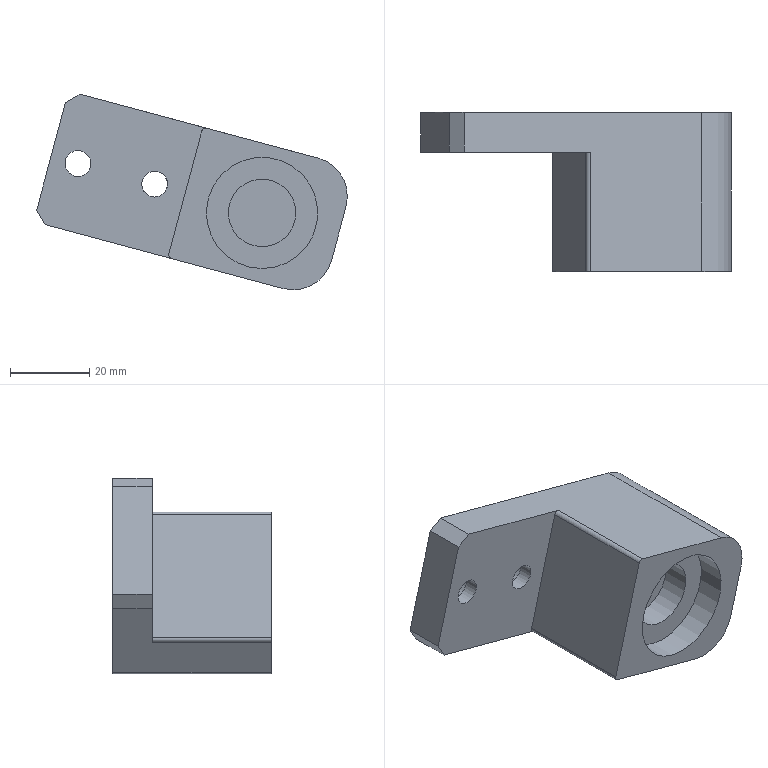Part | NX | 1 solid | 24 faces | box 78.22 x 40 x 49.229 mm | volume 57101 mm3 | plane 14 | cylinder 10 | commonest cylinder face diameters 2 x2 6.5 x2 11 x2 20 x2 17 x1 28.04 x1
STEP:
#1=CARTESIAN_POINT('',(554.778,70.097,-14.611));
#2=VERTEX_POINT('',#1);
#3=CARTESIAN_POINT('',(554.778,70.097,-0.5914));
#4=DIRECTION('',(0.,1.,0.));
#5=DIRECTION('',(0.000000051,0.,-1.));
#6=AXIS2_PLACEMENT_3D('',#3,#4,#5);
#7=CIRCLE('',#6,14.02);
#8=EDGE_CURVE('',#2,#2,#7,.T.);
#9=ORIENTED_EDGE('',*,*,#8,.F.);
#10=EDGE_LOOP('',(#9));
#11=FACE_BOUND('',#10,.T.);
#12=CARTESIAN_POINT('',(554.778,70.097,7.909));
#13=VERTEX_POINT('',#12);
#14=CARTESIAN_POINT('',(554.778,70.097,-0.5914));
#15=DIRECTION('',(0.,1.,0.));
#16=DIRECTION('',(0.,0.,1.));
#17=AXIS2_PLACEMENT_3D('',#14,#15,#16);
#18=CIRCLE('',#17,8.5);
#19=EDGE_CURVE('',#13,#13,#18,.T.);
#20=ORIENTED_EDGE('',*,*,#19,.T.);
#21=EDGE_LOOP('',(#20));
#22=FACE_BOUND('',#21,.T.);
#23=CARTESIAN_POINT('',(554.778,70.097,-0.5914));
#24=DIRECTION('',(0.,1.,0.));
#25=DIRECTION('',(0.9659,0.,-0.2588));
#26=AXIS2_PLACEMENT_3D('',#23,#24,#25);
#27=PLANE('',#26);
#28=ADVANCED_FACE('',(#11,#22),#27,.F.);
#29=CARTESIAN_POINT('',(508.413,103.097,17.332));
#30=VERTEX_POINT('',#29);
#31=CARTESIAN_POINT('',(508.413,103.097,11.832));
#32=DIRECTION('',(0.,1.,0.));
#33=DIRECTION('',(0.,0.,1.));
#34=AXIS2_PLACEMENT_3D('',#31,#32,#33);
#35=CIRCLE('',#34,5.5);
#36=EDGE_CURVE('',#30,#30,#35,.T.);
#37=ORIENTED_EDGE('',*,*,#36,.F.);
#38=EDGE_LOOP('',(#37));
#39=FACE_BOUND('',#38,.T.);
#40=CARTESIAN_POINT('',(527.732,103.097,12.156));
#41=VERTEX_POINT('',#40);
#42=CARTESIAN_POINT('',(527.732,103.097,6.656));
#43=DIRECTION('',(0.,1.,0.));
#44=DIRECTION('',(0.,0.,1.));
#45=AXIS2_PLACEMENT_3D('',#42,#43,#44);
#46=CIRCLE('',#45,5.5);
#47=EDGE_CURVE('',#41,#41,#46,.T.);
#48=ORIENTED_EDGE('',*,*,#47,.F.);
#49=EDGE_LOOP('',(#48));
#50=FACE_BOUND('',#49,.T.);
#51=CARTESIAN_POINT('',(498.028,103.097,0.1207));
#52=VERTEX_POINT('',#51);
#53=CARTESIAN_POINT('',(500.15,103.097,-3.554));
#54=VERTEX_POINT('',#53);
#55=CARTESIAN_POINT('',(500.15,103.097,-3.554));
#56=DIRECTION('',(0.5,0.,-0.866));
#57=VECTOR('',#56,1000.);
#58=LINE('',#55,#57);
#59=EDGE_CURVE('',#52,#54,#58,.T.);
#60=ORIENTED_EDGE('',*,*,#59,.F.);
#61=CARTESIAN_POINT('',(505.275,103.097,27.167));
#62=VERTEX_POINT('',#61);
#63=CARTESIAN_POINT('',(501.652,103.097,13.644));
#64=DIRECTION('',(0.2588,0.,0.9659));
#65=VECTOR('',#64,1000.);
#66=LINE('',#63,#65);
#67=EDGE_CURVE('',#52,#62,#66,.T.);
#68=ORIENTED_EDGE('',*,*,#67,.T.);
#69=CARTESIAN_POINT('',(508.95,103.097,29.288));
#70=VERTEX_POINT('',#69);
#71=CARTESIAN_POINT('',(505.275,103.097,27.167));
#72=DIRECTION('',(-0.866,0.,-0.5));
#73=VECTOR('',#72,1000.);
#74=LINE('',#71,#73);
#75=EDGE_CURVE('',#70,#62,#74,.T.);
#76=ORIENTED_EDGE('',*,*,#75,.F.);
#77=CARTESIAN_POINT('',(568.837,103.097,13.241));
#78=VERTEX_POINT('',#77);
#79=CARTESIAN_POINT('',(342.81,103.097,73.805));
#80=DIRECTION('',(-0.9659,0.,0.2588));
#81=VECTOR('',#80,1000.);
#82=LINE('',#79,#81);
#83=EDGE_CURVE('',#78,#70,#82,.T.);
#84=ORIENTED_EDGE('',*,*,#83,.F.);
#85=CARTESIAN_POINT('',(575.908,103.097,0.9937));
#86=VERTEX_POINT('',#85);
#87=CARTESIAN_POINT('',(566.249,103.097,3.582));
#88=DIRECTION('',(0.,1.,0.));
#89=DIRECTION('',(0.,0.,1.));
#90=AXIS2_PLACEMENT_3D('',#87,#88,#89);
#91=CIRCLE('',#90,10.);
#92=EDGE_CURVE('',#86,#78,#91,.F.);
#93=ORIENTED_EDGE('',*,*,#92,.F.);
#94=CARTESIAN_POINT('',(572.285,103.097,-12.529));
#95=VERTEX_POINT('',#94);
#96=CARTESIAN_POINT('',(572.802,103.097,-10.597));
#97=DIRECTION('',(0.2588,0.,0.9659));
#98=VECTOR('',#97,1000.);
#99=LINE('',#96,#98);
#100=EDGE_CURVE('',#95,#86,#99,.T.);
#101=ORIENTED_EDGE('',*,*,#100,.F.);
#102=CARTESIAN_POINT('',(560.037,103.097,-19.6));
#103=VERTEX_POINT('',#102);
#104=CARTESIAN_POINT('',(562.625,103.097,-9.941));
#105=DIRECTION('',(0.,1.,0.));
#106=DIRECTION('',(0.,0.,1.));
#107=AXIS2_PLACEMENT_3D('',#104,#105,#106);
#108=CIRCLE('',#107,10.);
#109=EDGE_CURVE('',#103,#95,#108,.F.);
#110=ORIENTED_EDGE('',*,*,#109,.F.);
#111=CARTESIAN_POINT('',(334.01,103.097,40.963));
#112=DIRECTION('',(0.9659,0.,-0.2588));
#113=VECTOR('',#112,1000.);
#114=LINE('',#111,#113);
#115=EDGE_CURVE('',#54,#103,#114,.T.);
#116=ORIENTED_EDGE('',*,*,#115,.F.);
#117=EDGE_LOOP('',(#60,#68,#76,#84,#93,#101,#110,#116));
#118=FACE_BOUND('',#117,.T.);
#119=CARTESIAN_POINT('',(334.528,103.097,42.895));
#120=DIRECTION('',(0.,1.,0.));
#121=DIRECTION('',(0.2588,0.,0.9659));
#122=AXIS2_PLACEMENT_3D('',#119,#120,#121);
#123=PLANE('',#122);
#124=ADVANCED_FACE('',(#39,#50,#118),#123,.T.);
#125=CARTESIAN_POINT('',(560.037,63.097,-19.6));
#126=VERTEX_POINT('',#125);
#127=CARTESIAN_POINT('',(560.037,78.097,-19.6));
#128=DIRECTION('',(0.,1.,0.));
#129=VECTOR('',#128,1000.);
#130=LINE('',#127,#129);
#131=EDGE_CURVE('',#126,#103,#130,.T.);
#132=ORIENTED_EDGE('',*,*,#131,.T.);
#133=ORIENTED_EDGE('',*,*,#109,.T.);
#134=CARTESIAN_POINT('',(572.285,63.097,-12.529));
#135=VERTEX_POINT('',#134);
#136=CARTESIAN_POINT('',(572.285,80.097,-12.529));
#137=DIRECTION('',(0.,-1.,0.));
#138=VECTOR('',#137,1000.);
#139=LINE('',#136,#138);
#140=EDGE_CURVE('',#95,#135,#139,.T.);
#141=ORIENTED_EDGE('',*,*,#140,.T.);
#142=CARTESIAN_POINT('',(562.625,63.097,-9.941));
#143=DIRECTION('',(0.,-1.,0.));
#144=DIRECTION('',(0.,0.,-1.));
#145=AXIS2_PLACEMENT_3D('',#142,#143,#144);
#146=CIRCLE('',#145,10.);
#147=EDGE_CURVE('',#135,#126,#146,.F.);
#148=ORIENTED_EDGE('',*,*,#147,.T.);
#149=EDGE_LOOP('',(#132,#133,#141,#148));
#150=FACE_BOUND('',#149,.T.);
#151=CARTESIAN_POINT('',(562.625,80.097,-9.941));
#152=DIRECTION('',(0.,1.,0.));
#153=DIRECTION('',(-0.9659,0.,0.2588));
#154=AXIS2_PLACEMENT_3D('',#151,#152,#153);
#155=CYLINDRICAL_SURFACE('',#154,10.);
#156=ADVANCED_FACE('',(#150),#155,.T.);
#157=CARTESIAN_POINT('',(532.025,63.097,-12.095));
#158=VERTEX_POINT('',#157);
#159=CARTESIAN_POINT('',(532.025,93.097,-12.095));
#160=VERTEX_POINT('',#159);
#161=CARTESIAN_POINT('',(532.025,93.097,-12.095));
#162=DIRECTION('',(0.,1.,0.));
#163=VECTOR('',#162,1000.);
#164=LINE('',#161,#163);
#165=EDGE_CURVE('',#158,#160,#164,.T.);
#166=ORIENTED_EDGE('',*,*,#165,.T.);
#167=CARTESIAN_POINT('',(500.15,93.097,-3.554));
#168=VERTEX_POINT('',#167);
#169=CARTESIAN_POINT('',(334.01,93.097,40.963));
#170=DIRECTION('',(0.9659,0.,-0.2588));
#171=VECTOR('',#170,1000.);
#172=LINE('',#169,#171);
#173=EDGE_CURVE('',#168,#160,#172,.T.);
#174=ORIENTED_EDGE('',*,*,#173,.F.);
#175=CARTESIAN_POINT('',(500.15,78.097,-3.554));
#176=DIRECTION('',(0.,-1.,0.));
#177=VECTOR('',#176,1000.);
#178=LINE('',#175,#177);
#179=EDGE_CURVE('',#54,#168,#178,.T.);
#180=ORIENTED_EDGE('',*,*,#179,.F.);
#181=ORIENTED_EDGE('',*,*,#115,.T.);
#182=ORIENTED_EDGE('',*,*,#131,.F.);
#183=CARTESIAN_POINT('',(334.01,63.097,40.963));
#184=DIRECTION('',(-0.9659,0.,0.2588));
#185=VECTOR('',#184,1000.);
#186=LINE('',#183,#185);
#187=EDGE_CURVE('',#126,#158,#186,.T.);
#188=ORIENTED_EDGE('',*,*,#187,.T.);
#189=EDGE_LOOP('',(#166,#174,#180,#181,#182,#188));
#190=FACE_BOUND('',#189,.T.);
#191=CARTESIAN_POINT('',(334.01,78.097,40.963));
#192=DIRECTION('',(-0.2588,0.,-0.9659));
#193=DIRECTION('',(0.,1.,0.));
#194=AXIS2_PLACEMENT_3D('',#191,#192,#193);
#195=PLANE('',#194);
#196=ADVANCED_FACE('',(#190),#195,.T.);
#197=ORIENTED_EDGE('',*,*,#165,.F.);
#198=CARTESIAN_POINT('',(531.318,63.097,-10.87));
#199=VERTEX_POINT('',#198);
#200=CARTESIAN_POINT('',(532.284,63.097,-11.129));
#201=DIRECTION('',(0.,-1.,0.));
#202=DIRECTION('',(0.,0.,-1.));
#203=AXIS2_PLACEMENT_3D('',#200,#201,#202);
#204=CIRCLE('',#203,1.);
#205=EDGE_CURVE('',#158,#199,#204,.F.);
#206=ORIENTED_EDGE('',*,*,#205,.T.);
#207=CARTESIAN_POINT('',(531.318,93.097,-10.87));
#208=VERTEX_POINT('',#207);
#209=CARTESIAN_POINT('',(531.318,63.097,-10.87));
#210=DIRECTION('',(0.,-1.,0.));
#211=VECTOR('',#210,1000.);
#212=LINE('',#209,#211);
#213=EDGE_CURVE('',#208,#199,#212,.T.);
#214=ORIENTED_EDGE('',*,*,#213,.F.);
#215=CARTESIAN_POINT('',(532.284,93.097,-11.129));
#216=DIRECTION('',(0.,1.,0.));
#217=DIRECTION('',(0.000000051,0.,-1.));
#218=AXIS2_PLACEMENT_3D('',#215,#216,#217);
#219=CIRCLE('',#218,1.);
#220=EDGE_CURVE('',#160,#208,#219,.T.);
#221=ORIENTED_EDGE('',*,*,#220,.F.);
#222=EDGE_LOOP('',(#197,#206,#214,#221));
#223=FACE_BOUND('',#222,.T.);
#224=CARTESIAN_POINT('',(532.284,70.097,-11.129));
#225=DIRECTION('',(0.,1.,0.));
#226=DIRECTION('',(0.000000051,0.,-1.));
#227=AXIS2_PLACEMENT_3D('',#224,#225,#226);
#228=CYLINDRICAL_SURFACE('',#227,1.);
#229=ADVANCED_FACE('',(#223),#228,.T.);
#230=CARTESIAN_POINT('',(539.6,63.097,20.04));
#231=VERTEX_POINT('',#230);
#232=CARTESIAN_POINT('',(535.459,63.097,4.585));
#233=DIRECTION('',(-0.2588,0.,-0.9659));
#234=VECTOR('',#233,1000.);
#235=LINE('',#232,#234);
#236=EDGE_CURVE('',#231,#199,#235,.T.);
#237=ORIENTED_EDGE('',*,*,#236,.F.);
#238=CARTESIAN_POINT('',(539.6,93.097,20.04));
#239=VERTEX_POINT('',#238);
#240=CARTESIAN_POINT('',(539.6,93.097,20.04));
#241=DIRECTION('',(0.,1.,0.));
#242=VECTOR('',#241,1000.);
#243=LINE('',#240,#242);
#244=EDGE_CURVE('',#231,#239,#243,.T.);
#245=ORIENTED_EDGE('',*,*,#244,.T.);
#246=CARTESIAN_POINT('',(535.459,93.097,4.585));
#247=DIRECTION('',(-0.2588,0.,-0.9659));
#248=VECTOR('',#247,1000.);
#249=LINE('',#246,#248);
#250=EDGE_CURVE('',#239,#208,#249,.T.);
#251=ORIENTED_EDGE('',*,*,#250,.T.);
#252=ORIENTED_EDGE('',*,*,#213,.T.);
#253=EDGE_LOOP('',(#237,#245,#251,#252));
#254=FACE_BOUND('',#253,.T.);
#255=CARTESIAN_POINT('',(535.459,70.097,4.585));
#256=DIRECTION('',(0.9659,0.,-0.2588));
#257=DIRECTION('',(0.2588,0.,0.9659));
#258=AXIS2_PLACEMENT_3D('',#255,#256,#257);
#259=PLANE('',#258);
#260=ADVANCED_FACE('',(#254),#259,.F.);
#261=ORIENTED_EDGE('',*,*,#244,.F.);
#262=CARTESIAN_POINT('',(540.825,63.097,20.747));
#263=VERTEX_POINT('',#262);
#264=CARTESIAN_POINT('',(540.566,63.097,19.781));
#265=DIRECTION('',(0.,-1.,0.));
#266=DIRECTION('',(0.,0.,-1.));
#267=AXIS2_PLACEMENT_3D('',#264,#265,#266);
#268=CIRCLE('',#267,1.);
#269=EDGE_CURVE('',#231,#263,#268,.F.);
#270=ORIENTED_EDGE('',*,*,#269,.T.);
#271=CARTESIAN_POINT('',(540.825,93.097,20.747));
#272=VERTEX_POINT('',#271);
#273=CARTESIAN_POINT('',(540.825,63.097,20.747));
#274=DIRECTION('',(0.,-1.,0.));
#275=VECTOR('',#274,1000.);
#276=LINE('',#273,#275);
#277=EDGE_CURVE('',#272,#263,#276,.T.);
#278=ORIENTED_EDGE('',*,*,#277,.F.);
#279=CARTESIAN_POINT('',(540.566,93.097,19.781));
#280=DIRECTION('',(0.,1.,0.));
#281=DIRECTION('',(0.000000051,0.,-1.));
#282=AXIS2_PLACEMENT_3D('',#279,#280,#281);
#283=CIRCLE('',#282,1.);
#284=EDGE_CURVE('',#239,#272,#283,.T.);
#285=ORIENTED_EDGE('',*,*,#284,.F.);
#286=EDGE_LOOP('',(#261,#270,#278,#285));
#287=FACE_BOUND('',#286,.T.);
#288=CARTESIAN_POINT('',(540.566,78.097,19.781));
#289=DIRECTION('',(0.,1.,0.));
#290=DIRECTION('',(0.000000051,0.,-1.));
#291=AXIS2_PLACEMENT_3D('',#288,#289,#290);
#292=CYLINDRICAL_SURFACE('',#291,1.);
#293=ADVANCED_FACE('',(#287),#292,.T.);
#294=CARTESIAN_POINT('',(508.95,93.097,29.288));
#295=VERTEX_POINT('',#294);
#296=CARTESIAN_POINT('',(342.81,93.097,73.805));
#297=DIRECTION('',(-0.9659,0.,0.2588));
#298=VECTOR('',#297,1000.);
#299=LINE('',#296,#298);
#300=EDGE_CURVE('',#272,#295,#299,.T.);
#301=ORIENTED_EDGE('',*,*,#300,.F.);
#302=ORIENTED_EDGE('',*,*,#277,.T.);
#303=CARTESIAN_POINT('',(568.837,63.097,13.241));
#304=VERTEX_POINT('',#303);
#305=CARTESIAN_POINT('',(342.81,63.097,73.805));
#306=DIRECTION('',(0.9659,0.,-0.2588));
#307=VECTOR('',#306,1000.);
#308=LINE('',#305,#307);
#309=EDGE_CURVE('',#263,#304,#308,.T.);
#310=ORIENTED_EDGE('',*,*,#309,.T.);
#311=CARTESIAN_POINT('',(568.837,78.097,13.241));
#312=DIRECTION('',(0.,-1.,0.));
#313=VECTOR('',#312,1000.);
#314=LINE('',#311,#313);
#315=EDGE_CURVE('',#78,#304,#314,.T.);
#316=ORIENTED_EDGE('',*,*,#315,.F.);
#317=ORIENTED_EDGE('',*,*,#83,.T.);
#318=CARTESIAN_POINT('',(508.95,70.097,29.288));
#319=DIRECTION('',(0.,1.,0.));
#320=VECTOR('',#319,1000.);
#321=LINE('',#318,#320);
#322=EDGE_CURVE('',#295,#70,#321,.T.);
#323=ORIENTED_EDGE('',*,*,#322,.F.);
#324=EDGE_LOOP('',(#301,#302,#310,#316,#317,#323));
#325=FACE_BOUND('',#324,.T.);
#326=CARTESIAN_POINT('',(342.81,78.097,73.805));
#327=DIRECTION('',(0.2588,0.,0.9659));
#328=DIRECTION('',(0.,-1.,0.));
#329=AXIS2_PLACEMENT_3D('',#326,#327,#328);
#330=PLANE('',#329);
#331=ADVANCED_FACE('',(#325),#330,.T.);
#332=CARTESIAN_POINT('',(575.908,63.097,0.9937));
#333=VERTEX_POINT('',#332);
#334=CARTESIAN_POINT('',(575.908,80.097,0.9937));
#335=DIRECTION('',(0.,1.,0.));
#336=VECTOR('',#335,1000.);
#337=LINE('',#334,#336);
#338=EDGE_CURVE('',#333,#86,#337,.T.);
#339=ORIENTED_EDGE('',*,*,#338,.T.);
#340=ORIENTED_EDGE('',*,*,#92,.T.);
#341=ORIENTED_EDGE('',*,*,#315,.T.);
#342=CARTESIAN_POINT('',(566.249,63.097,3.582));
#343=DIRECTION('',(0.,-1.,0.));
#344=DIRECTION('',(0.,0.,-1.));
#345=AXIS2_PLACEMENT_3D('',#342,#343,#344);
#346=CIRCLE('',#345,10.);
#347=EDGE_CURVE('',#304,#333,#346,.F.);
#348=ORIENTED_EDGE('',*,*,#347,.T.);
#349=EDGE_LOOP('',(#339,#340,#341,#348));
#350=FACE_BOUND('',#349,.T.);
#351=CARTESIAN_POINT('',(566.249,80.097,3.582));
#352=DIRECTION('',(0.,-1.,0.));
#353=DIRECTION('',(0.9659,0.,-0.2588));
#354=AXIS2_PLACEMENT_3D('',#351,#352,#353);
#355=CYLINDRICAL_SURFACE('',#354,10.);
#356=ADVANCED_FACE('',(#350),#355,.T.);
#357=ORIENTED_EDGE('',*,*,#140,.F.);
#358=ORIENTED_EDGE('',*,*,#100,.T.);
#359=ORIENTED_EDGE('',*,*,#338,.F.);
#360=CARTESIAN_POINT('',(572.802,63.097,-10.597));
#361=DIRECTION('',(-0.2588,0.,-0.9659));
#362=VECTOR('',#361,1000.);
#363=LINE('',#360,#362);
#364=EDGE_CURVE('',#333,#135,#363,.T.);
#365=ORIENTED_EDGE('',*,*,#364,.T.);
#366=EDGE_LOOP('',(#357,#358,#359,#365));
#367=FACE_BOUND('',#366,.T.);
#368=CARTESIAN_POINT('',(572.802,80.097,-10.597));
#369=DIRECTION('',(0.9659,0.,-0.2588));
#370=DIRECTION('',(0.,-1.,0.));
#371=AXIS2_PLACEMENT_3D('',#368,#369,#370);
#372=PLANE('',#371);
#373=ADVANCED_FACE('',(#367),#372,.T.);
#374=CARTESIAN_POINT('',(527.732,96.597,1.156));
#375=VERTEX_POINT('',#374);
#376=CARTESIAN_POINT('',(527.732,96.597,6.656));
#377=DIRECTION('',(0.,1.,0.));
#378=DIRECTION('',(0.,0.,-1.));
#379=AXIS2_PLACEMENT_3D('',#376,#377,#378);
#380=CIRCLE('',#379,5.5);
#381=EDGE_CURVE('',#375,#375,#380,.T.);
#382=ORIENTED_EDGE('',*,*,#381,.F.);
#383=EDGE_LOOP('',(#382));
#384=FACE_BOUND('',#383,.T.);
#385=ORIENTED_EDGE('',*,*,#47,.T.);
#386=EDGE_LOOP('',(#385));
#387=FACE_BOUND('',#386,.T.);
#388=CARTESIAN_POINT('',(527.732,103.097,6.656));
#389=DIRECTION('',(0.,-1.,0.));
#390=DIRECTION('',(-0.2588,0.,-0.9659));
#391=AXIS2_PLACEMENT_3D('',#388,#389,#390);
#392=CYLINDRICAL_SURFACE('',#391,5.5);
#393=ADVANCED_FACE('',(#384,#387),#392,.F.);
#394=CARTESIAN_POINT('',(506.99,96.597,6.519));
#395=VERTEX_POINT('',#394);
#396=CARTESIAN_POINT('',(508.413,96.597,11.832));
#397=DIRECTION('',(0.,1.,0.));
#398=DIRECTION('',(-0.2588,0.,-0.9659));
#399=AXIS2_PLACEMENT_3D('',#396,#397,#398);
#400=CIRCLE('',#399,5.5);
#401=EDGE_CURVE('',#395,#395,#400,.T.);
#402=ORIENTED_EDGE('',*,*,#401,.F.);
#403=EDGE_LOOP('',(#402));
#404=FACE_BOUND('',#403,.T.);
#405=ORIENTED_EDGE('',*,*,#36,.T.);
#406=EDGE_LOOP('',(#405));
#407=FACE_BOUND('',#406,.T.);
#408=CARTESIAN_POINT('',(508.413,103.097,11.832));
#409=DIRECTION('',(0.,-1.,0.));
#410=DIRECTION('',(-0.2588,0.,-0.9659));
#411=AXIS2_PLACEMENT_3D('',#408,#409,#410);
#412=CYLINDRICAL_SURFACE('',#411,5.5);
#413=ADVANCED_FACE('',(#404,#407),#412,.F.);
#414=ORIENTED_EDGE('',*,*,#381,.T.);
#415=EDGE_LOOP('',(#414));
#416=FACE_BOUND('',#415,.T.);
#417=CARTESIAN_POINT('',(527.732,96.597,3.406));
#418=VERTEX_POINT('',#417);
#419=CARTESIAN_POINT('',(527.732,96.597,6.656));
#420=DIRECTION('',(0.,1.,0.));
#421=DIRECTION('',(0.,0.,-1.));
#422=AXIS2_PLACEMENT_3D('',#419,#420,#421);
#423=CIRCLE('',#422,3.25);
#424=EDGE_CURVE('',#418,#418,#423,.T.);
#425=ORIENTED_EDGE('',*,*,#424,.F.);
#426=EDGE_LOOP('',(#425));
#427=FACE_BOUND('',#426,.T.);
#428=CARTESIAN_POINT('',(508.413,96.597,11.832));
#429=DIRECTION('',(0.,-1.,0.));
#430=DIRECTION('',(-0.2588,0.,-0.9659));
#431=AXIS2_PLACEMENT_3D('',#428,#429,#430);
#432=PLANE('',#431);
#433=ADVANCED_FACE('',(#416,#427),#432,.F.);
#434=ORIENTED_EDGE('',*,*,#401,.T.);
#435=EDGE_LOOP('',(#434));
#436=FACE_BOUND('',#435,.T.);
#437=CARTESIAN_POINT('',(507.572,96.597,8.693));
#438=VERTEX_POINT('',#437);
#439=CARTESIAN_POINT('',(508.413,96.597,11.832));
#440=DIRECTION('',(0.,1.,0.));
#441=DIRECTION('',(-0.2588,0.,-0.9659));
#442=AXIS2_PLACEMENT_3D('',#439,#440,#441);
#443=CIRCLE('',#442,3.25);
#444=EDGE_CURVE('',#438,#438,#443,.T.);
#445=ORIENTED_EDGE('',*,*,#444,.F.);
#446=EDGE_LOOP('',(#445));
#447=FACE_BOUND('',#446,.T.);
#448=CARTESIAN_POINT('',(508.413,96.597,11.832));
#449=DIRECTION('',(0.,-1.,0.));
#450=DIRECTION('',(-0.2588,0.,-0.9659));
#451=AXIS2_PLACEMENT_3D('',#448,#449,#450);
#452=PLANE('',#451);
#453=ADVANCED_FACE('',(#436,#447),#452,.F.);
#454=CARTESIAN_POINT('',(528.573,93.097,9.795));
#455=VERTEX_POINT('',#454);
#456=CARTESIAN_POINT('',(527.732,93.097,6.656));
#457=DIRECTION('',(0.,-1.,0.));
#458=DIRECTION('',(0.2588,0.,0.9659));
#459=AXIS2_PLACEMENT_3D('',#456,#457,#458);
#460=CIRCLE('',#459,3.25);
#461=EDGE_CURVE('',#455,#455,#460,.T.);
#462=ORIENTED_EDGE('',*,*,#461,.T.);
#463=EDGE_LOOP('',(#462));
#464=FACE_BOUND('',#463,.T.);
#465=ORIENTED_EDGE('',*,*,#424,.T.);
#466=EDGE_LOOP('',(#465));
#467=FACE_BOUND('',#466,.T.);
#468=CARTESIAN_POINT('',(527.732,33.097,6.656));
#469=DIRECTION('',(0.,-1.,0.));
#470=DIRECTION('',(-0.2588,0.,-0.9659));
#471=AXIS2_PLACEMENT_3D('',#468,#469,#470);
#472=CYLINDRICAL_SURFACE('',#471,3.25);
#473=ADVANCED_FACE('',(#464,#467),#472,.F.);
#474=CARTESIAN_POINT('',(509.254,93.097,14.971));
#475=VERTEX_POINT('',#474);
#476=CARTESIAN_POINT('',(508.413,93.097,11.832));
#477=DIRECTION('',(0.,-1.,0.));
#478=DIRECTION('',(0.2588,0.,0.9659));
#479=AXIS2_PLACEMENT_3D('',#476,#477,#478);
#480=CIRCLE('',#479,3.25);
#481=EDGE_CURVE('',#475,#475,#480,.T.);
#482=ORIENTED_EDGE('',*,*,#481,.T.);
#483=EDGE_LOOP('',(#482));
#484=FACE_BOUND('',#483,.T.);
#485=ORIENTED_EDGE('',*,*,#444,.T.);
#486=EDGE_LOOP('',(#485));
#487=FACE_BOUND('',#486,.T.);
#488=CARTESIAN_POINT('',(508.413,33.097,11.832));
#489=DIRECTION('',(0.,-1.,0.));
#490=DIRECTION('',(-0.2588,0.,-0.9659));
#491=AXIS2_PLACEMENT_3D('',#488,#489,#490);
#492=CYLINDRICAL_SURFACE('',#491,3.25);
#493=ADVANCED_FACE('',(#484,#487),#492,.F.);
#494=ORIENTED_EDGE('',*,*,#67,.F.);
#495=CARTESIAN_POINT('',(498.028,93.097,0.1207));
#496=VERTEX_POINT('',#495);
#497=CARTESIAN_POINT('',(498.028,70.097,0.1207));
#498=DIRECTION('',(0.,1.,0.));
#499=VECTOR('',#498,1000.);
#500=LINE('',#497,#499);
#501=EDGE_CURVE('',#496,#52,#500,.T.);
#502=ORIENTED_EDGE('',*,*,#501,.F.);
#503=CARTESIAN_POINT('',(505.275,93.097,27.167));
#504=VERTEX_POINT('',#503);
#505=CARTESIAN_POINT('',(501.652,93.097,13.644));
#506=DIRECTION('',(0.2588,0.,0.9659));
#507=VECTOR('',#506,1000.);
#508=LINE('',#505,#507);
#509=EDGE_CURVE('',#504,#496,#508,.F.);
#510=ORIENTED_EDGE('',*,*,#509,.F.);
#511=CARTESIAN_POINT('',(505.275,70.097,27.167));
#512=DIRECTION('',(0.,-1.,0.));
#513=VECTOR('',#512,1000.);
#514=LINE('',#511,#513);
#515=EDGE_CURVE('',#62,#504,#514,.T.);
#516=ORIENTED_EDGE('',*,*,#515,.F.);
#517=EDGE_LOOP('',(#494,#502,#510,#516));
#518=FACE_BOUND('',#517,.T.);
#519=CARTESIAN_POINT('',(501.652,70.097,13.644));
#520=DIRECTION('',(0.9659,0.,-0.2588));
#521=DIRECTION('',(0.2588,0.,0.9659));
#522=AXIS2_PLACEMENT_3D('',#519,#520,#521);
#523=PLANE('',#522);
#524=ADVANCED_FACE('',(#518),#523,.F.);
#525=ORIENTED_EDGE('',*,*,#322,.T.);
#526=ORIENTED_EDGE('',*,*,#75,.T.);
#527=ORIENTED_EDGE('',*,*,#515,.T.);
#528=CARTESIAN_POINT('',(505.275,93.097,27.167));
#529=DIRECTION('',(-0.866,0.,-0.5));
#530=VECTOR('',#529,1000.);
#531=LINE('',#528,#530);
#532=EDGE_CURVE('',#295,#504,#531,.T.);
#533=ORIENTED_EDGE('',*,*,#532,.F.);
#534=EDGE_LOOP('',(#525,#526,#527,#533));
#535=FACE_BOUND('',#534,.T.);
#536=CARTESIAN_POINT('',(505.275,70.097,27.167));
#537=DIRECTION('',(-0.5,0.,0.866));
#538=DIRECTION('',(0.866,0.,0.5));
#539=AXIS2_PLACEMENT_3D('',#536,#537,#538);
#540=PLANE('',#539);
#541=ADVANCED_FACE('',(#535),#540,.T.);
#542=ORIENTED_EDGE('',*,*,#173,.T.);
#543=ORIENTED_EDGE('',*,*,#220,.T.);
#544=ORIENTED_EDGE('',*,*,#250,.F.);
#545=ORIENTED_EDGE('',*,*,#284,.T.);
#546=ORIENTED_EDGE('',*,*,#300,.T.);
#547=ORIENTED_EDGE('',*,*,#532,.T.);
#548=ORIENTED_EDGE('',*,*,#509,.T.);
#549=CARTESIAN_POINT('',(500.15,93.097,-3.554));
#550=DIRECTION('',(0.5,0.,-0.866));
#551=VECTOR('',#550,1000.);
#552=LINE('',#549,#551);
#553=EDGE_CURVE('',#496,#168,#552,.T.);
#554=ORIENTED_EDGE('',*,*,#553,.T.);
#555=EDGE_LOOP('',(#542,#543,#544,#545,#546,#547,#548,#554));
#556=FACE_BOUND('',#555,.T.);
#557=ORIENTED_EDGE('',*,*,#481,.F.);
#558=EDGE_LOOP('',(#557));
#559=FACE_BOUND('',#558,.T.);
#560=ORIENTED_EDGE('',*,*,#461,.F.);
#561=EDGE_LOOP('',(#560));
#562=FACE_BOUND('',#561,.T.);
#563=CARTESIAN_POINT('',(542.704,93.097,2.644));
#564=DIRECTION('',(0.,1.,0.));
#565=DIRECTION('',(0.2588,0.,0.9659));
#566=AXIS2_PLACEMENT_3D('',#563,#564,#565);
#567=PLANE('',#566);
#568=ADVANCED_FACE('',(#556,#559,#562),#567,.F.);
#569=ORIENTED_EDGE('',*,*,#501,.T.);
#570=ORIENTED_EDGE('',*,*,#59,.T.);
#571=ORIENTED_EDGE('',*,*,#179,.T.);
#572=ORIENTED_EDGE('',*,*,#553,.F.);
#573=EDGE_LOOP('',(#569,#570,#571,#572));
#574=FACE_BOUND('',#573,.T.);
#575=CARTESIAN_POINT('',(500.15,78.097,-3.554));
#576=DIRECTION('',(-0.866,0.,-0.5));
#577=DIRECTION('',(-0.5,0.,0.866));
#578=AXIS2_PLACEMENT_3D('',#575,#576,#577);
#579=PLANE('',#578);
#580=ADVANCED_FACE('',(#574),#579,.T.);
#581=CARTESIAN_POINT('',(554.778,63.097,-14.611));
#582=VERTEX_POINT('',#581);
#583=CARTESIAN_POINT('',(554.778,63.097,-0.5914));
#584=DIRECTION('',(0.,-1.,0.));
#585=DIRECTION('',(0.,0.,-1.));
#586=AXIS2_PLACEMENT_3D('',#583,#584,#585);
#587=CIRCLE('',#586,14.02);
#588=EDGE_CURVE('',#582,#582,#587,.T.);
#589=ORIENTED_EDGE('',*,*,#588,.F.);
#590=EDGE_LOOP('',(#589));
#591=FACE_BOUND('',#590,.T.);
#592=ORIENTED_EDGE('',*,*,#147,.F.);
#593=ORIENTED_EDGE('',*,*,#364,.F.);
#594=ORIENTED_EDGE('',*,*,#347,.F.);
#595=ORIENTED_EDGE('',*,*,#309,.F.);
#596=ORIENTED_EDGE('',*,*,#269,.F.);
#597=ORIENTED_EDGE('',*,*,#236,.T.);
#598=ORIENTED_EDGE('',*,*,#205,.F.);
#599=ORIENTED_EDGE('',*,*,#187,.F.);
#600=EDGE_LOOP('',(#592,#593,#594,#595,#596,#597,#598,#599));
#601=FACE_BOUND('',#600,.T.);
#602=CARTESIAN_POINT('',(99.499,63.097,116.224));
#603=DIRECTION('',(0.,-1.,0.));
#604=DIRECTION('',(-0.9659,0.,0.2588));
#605=AXIS2_PLACEMENT_3D('',#602,#603,#604);
#606=PLANE('',#605);
#607=ADVANCED_FACE('',(#591,#601),#606,.T.);
#608=ORIENTED_EDGE('',*,*,#8,.T.);
#609=EDGE_LOOP('',(#608));
#610=FACE_BOUND('',#609,.T.);
#611=ORIENTED_EDGE('',*,*,#588,.T.);
#612=EDGE_LOOP('',(#611));
#613=FACE_BOUND('',#612,.T.);
#614=CARTESIAN_POINT('',(554.778,70.097,-0.5914));
#615=DIRECTION('',(0.,-1.,0.));
#616=DIRECTION('',(-0.2588,0.,-0.9659));
#617=AXIS2_PLACEMENT_3D('',#614,#615,#616);
#618=CYLINDRICAL_SURFACE('',#617,14.02);
#619=ADVANCED_FACE('',(#610,#613),#618,.F.);
#620=CARTESIAN_POINT('',(554.778,77.097,-9.091));
#621=VERTEX_POINT('',#620);
#622=CARTESIAN_POINT('',(554.778,77.097,-0.5914));
#623=DIRECTION('',(0.,-1.,0.));
#624=DIRECTION('',(0.000000051,0.,-1.));
#625=AXIS2_PLACEMENT_3D('',#622,#623,#624);
#626=CIRCLE('',#625,8.5);
#627=EDGE_CURVE('',#621,#621,#626,.T.);
#628=ORIENTED_EDGE('',*,*,#627,.T.);
#629=EDGE_LOOP('',(#628));
#630=FACE_BOUND('',#629,.T.);
#631=CARTESIAN_POINT('',(554.778,77.097,-0.5914));
#632=DIRECTION('',(0.,1.,0.));
#633=DIRECTION('',(0.000000051,0.,-1.));
#634=AXIS2_PLACEMENT_3D('',#631,#632,#633);
#635=PLANE('',#634);
#636=ADVANCED_FACE('',(#630),#635,.F.);
#637=ORIENTED_EDGE('',*,*,#627,.F.);
#638=EDGE_LOOP('',(#637));
#639=FACE_BOUND('',#638,.T.);
#640=ORIENTED_EDGE('',*,*,#19,.F.);
#641=EDGE_LOOP('',(#640));
#642=FACE_BOUND('',#641,.T.);
#643=CARTESIAN_POINT('',(554.778,85.097,-0.5914));
#644=DIRECTION('',(0.,1.,0.));
#645=DIRECTION('',(0.2588,0.,0.9659));
#646=AXIS2_PLACEMENT_3D('',#643,#644,#645);
#647=CYLINDRICAL_SURFACE('',#646,8.5);
#648=ADVANCED_FACE('',(#639,#642),#647,.F.);
#649=CLOSED_SHELL('',(#28,#124,#156,#196,#229,#260,#293,#331,#356,#373,#393,#413,#433,#453,#473,#493,#524,#541,#568,#580,#607,#619,#636,#648));
#650=MANIFOLD_SOLID_BREP('',#649);
#651=(LENGTH_UNIT()NAMED_UNIT(*)SI_UNIT(.MILLI.,.METRE.));
#652=UNCERTAINTY_MEASURE_WITH_UNIT(LENGTH_MEASURE(0.00001),#651,'','');
#653=(NAMED_UNIT(*)PLANE_ANGLE_UNIT()SI_UNIT($,.RADIAN.));
#654=(NAMED_UNIT(*)SI_UNIT($,.STERADIAN.)SOLID_ANGLE_UNIT());
#655=(GEOMETRIC_REPRESENTATION_CONTEXT(3)GLOBAL_UNCERTAINTY_ASSIGNED_CONTEXT((#652))GLOBAL_UNIT_ASSIGNED_CONTEXT((#651,#653,#654))REPRESENTATION_CONTEXT('',''));
#656=ADVANCED_BREP_SHAPE_REPRESENTATION('',(#650),#655);